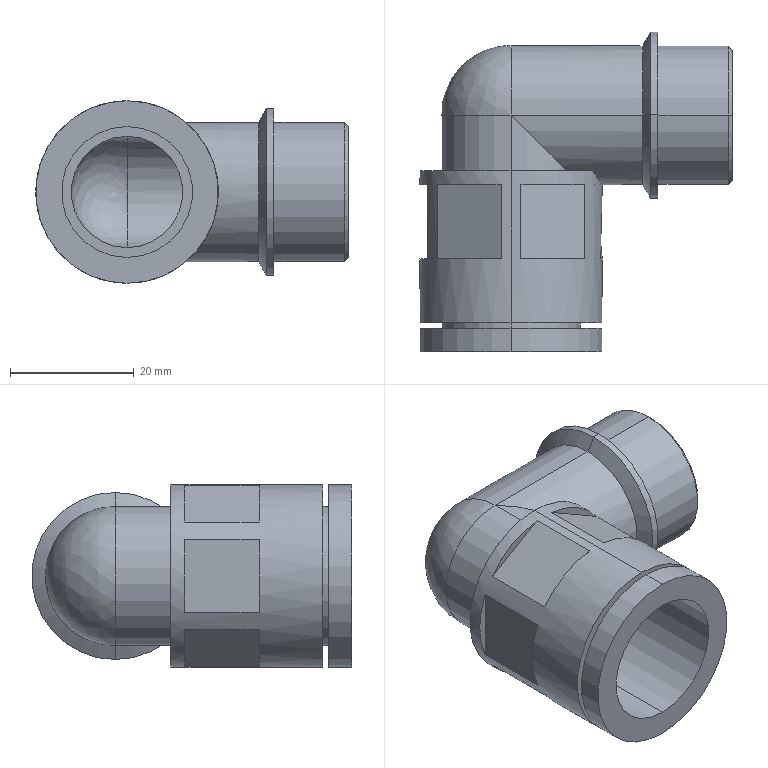Part | STEP file | 00177576_EZT_L-SCH.SCHL.VER._MKRL-16.5-PG-16 | 1 solid | 52 faces | box 50.5 x 51.75 x 29.5 mm | volume 15308 mm3 | plane 25 | cylinder 21 | cone 4 | spline 2 | commonest cylinder face diameters 22.5 x9 18 x4 29.5 x4 21.16 x2 27 x2